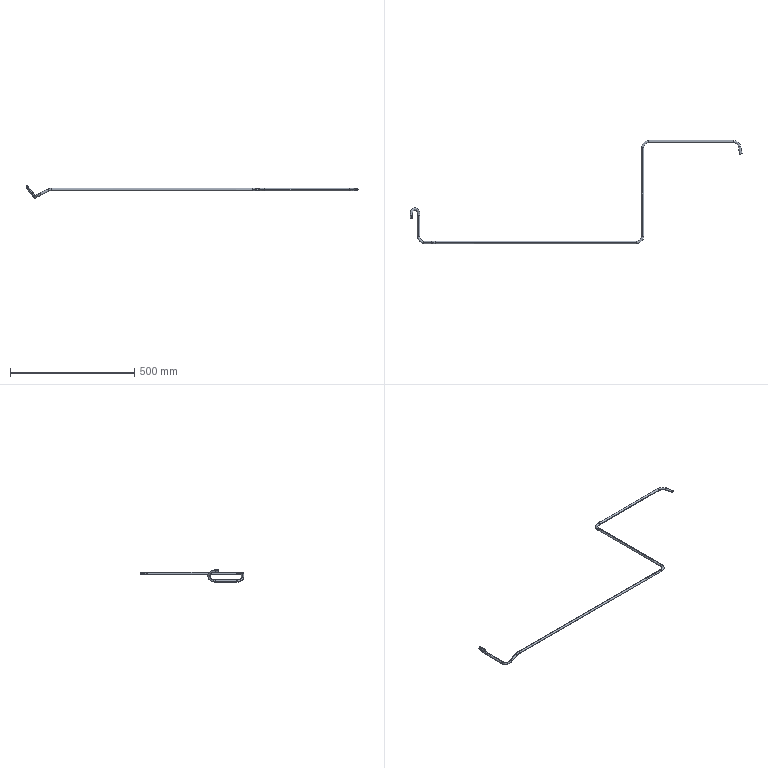Part | STEP file | copper tube 18_default_machined_ | 1 solid | 54 faces | box 1334 x 414.525 x 49.525 mm | volume 41948 mm3 | cylinder 28 | spline 24 | plane 2 | commonest cylinder face diameters 7.925 x14 9.525 x14